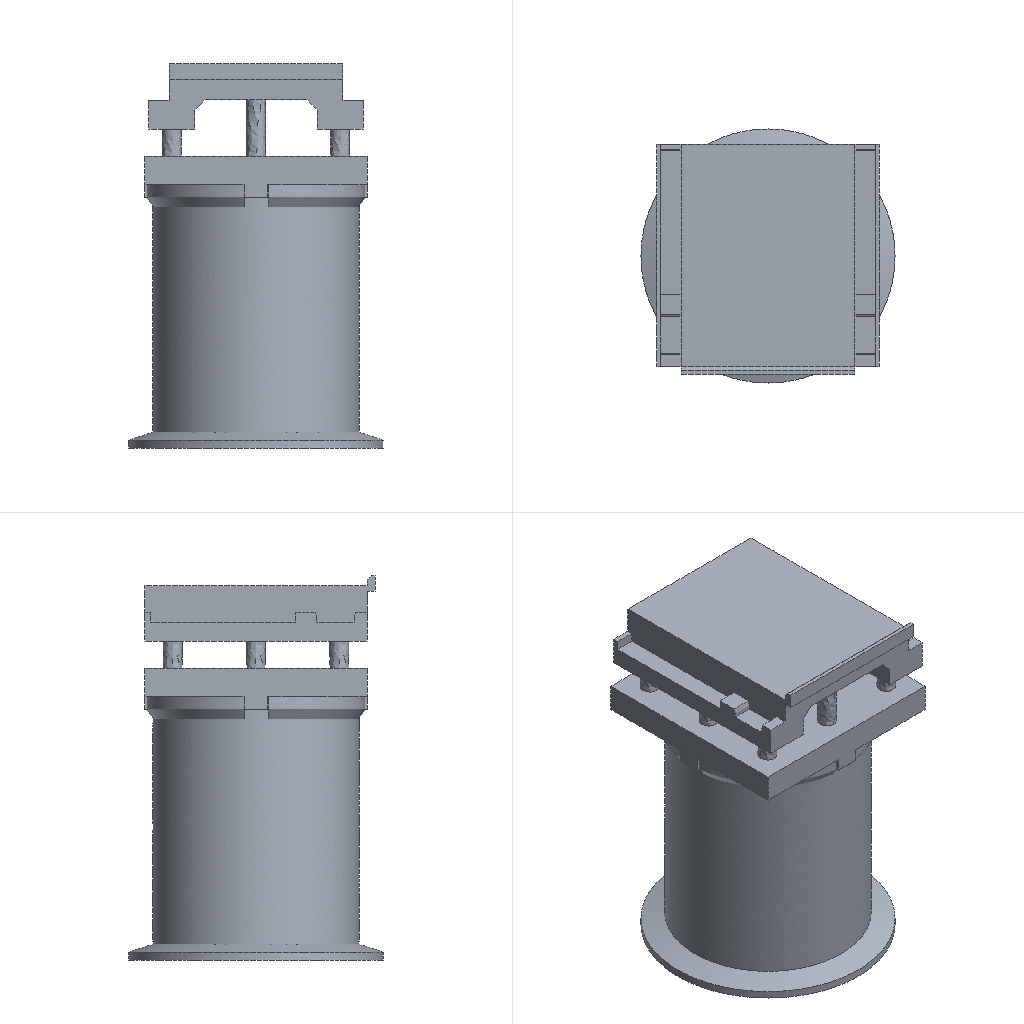Simulation study | ansys workbench
Ansys APDL input file, long lists of numbers shortened:
/batch
/config,noeldb,1     ! force off writing results to database
*get,_wallstrt,active,,time,wall
! ANSYS input file written by Workbench version 2022 R1
! File used for geometry attach:
/title,wbnew--____ (A5)
! ****** Begin Custom Load Command Snippet ******
/COM, ACT Extensions:
/COM,     LSDYNA, 2021.1
/COM,
! ****** End   Custom Load Command Snippet ******
*DIM,_wb_ProjectScratch_dir,string,248
_wb_ProjectScratch_dir(1) = ''
*DIM,_wb_SolverFiles_dir,string,248
_wb_SolverFiles_dir(1) = ''
*DIM,_wb_userfiles_dir,string,248
_wb_userfiles_dir(1) = ''
/com,--- Data in consistent MKS units. See Solving Units in the help system for more information.
/units,MKS
/nopr
/wb,file,start              !  signify a WB generated input file
/prep7
! Turn off shape checking because checks already performed inside WB mesher.
! See help system for more information.
SHPP,OFF,,NOWARN
/nolist
etcon,set             ! allow ANSYS to choose best KEYOP's for 180x elements, resets any applicable keyopt to MAPDL defaults
/com,*********** Nodes for the whole assembly ***********
nblock,3,,165333
(1i9,3e20.9e3)
        1    -4.091861413E+02     3.968814041E+01    -2.039000000E+01
! (150302 more lines like these left out)
-1
/wb,elem,start            !  set before creation of elements
/com,*********** Elements for Body 1 "a953f0-7" ***********
et,1,187
eblock,19,solid,,87505
(19i9)
        1        1        1        1        0        0        0        0       10        0        1    11820    23372    11975    23358    91085    91919    91082    91084
! (175009 more lines like these left out)
-1
/wb,elem,end               !  done creating elements
/com,*********** Send User Defined Coordinate System(s) ***********
csys,0
toffst,273.15,  ! Temperature offset from absolute zero
/com,*********** Set Reference Temperature ***********
tref,22.
/wb,mat,start              !  starting to send materials
/com,*********** Send Materials ***********
Temperature = 'TEMP' ! Temperature
MP,DENS,1,2300,	! kg m^-3
MP,ALPX,1,1.4e-05,	! C^-1
MP,C,1,780,	! J kg^-1 C^-1
MP,KXX,1,0.72,	! W m^-1 C^-1
MP,EX,1,30000000000,	! Pa
MP,NUXY,1,0.18,
/wb,mat,end                !  done sending materials
!************************* Model Summary ********************
!a953f0-7,	混凝土,	matid,	1
!************************* End Model Summary ********************
! get the diagonal of the bounding box. Needed later for other things
*get,_xmin,node,,mnloc,x
*get,_ymin,node,,mnloc,y
*get,_zmin,node,,mnloc,z
*get,_xmax,node,,mxloc,x
*get,_ymax,node,,mxloc,y
*get,_zmax,node,,mxloc,z
_ASMDIAG=(_xmax-_xmin)*(_xmax-_xmin)+(_ymax-_ymin)*(_ymax-_ymin)+(_zmax-_zmin)*(_zmax-_zmin)
_ASMDIAG=SQRT(_ASMDIAG)
/wb,contact,start          !  starting to send contact
/wb,contact,end            !  done creating contacts
/golist
/wb,load,start             !  starting to send loads
/com,*********** Fixed Supports ***********
CMBLOCK,_FIXEDSU,NODE,     7355
(8i10)
         1        96       121       122       123       124       125       126
! (919 more lines like these left out)
cmsel,s,_FIXEDSU
d,all,all
nsel,all
/com,*********** Define Force Using Surface Effect Elements ***********
local,12,0,0.,0.,0.,0.,0.,0.
csys,0
et,2,154
eblock,10,,,7449
(15i9)
   119600        2        2        2       12       15    11737       14       14    23478    23472       14    23468
! (7448 more lines like these left out)
-1
esel,s,type,,2
keyop,2,2,1                ! Apply load in local coordinate system
keyop,2,7,1                ! Use original area so load is constant in large deformation
esel,all
/gst,on,on
fini
*get,_numnode,node,0,count
*get,_numelem,elem,0,count
*get, _MAXELEMNUM, elem, 0, NUM, MAX
*get, _MAXNODENUM, node, 0, NUM, MAX
*get, _MAXELEMTYPE, etyp, 0, NUM, MAX
*get, _MAXREALCONST, real, 0, NUM, MAX
/go
/wb,load,end               !  done creating loads
/com,--- Number of total nodes = %_numnode%
/com,--- Number of contact elements = 7449
/com,--- Number of spring elements = 0
/com,--- Number of bearing elements = 0
/com,--- Number of solid elements = 87505
/com,--- Number of condensed parts = 0
/com,--- Number of total elements = %_numelem%
*get,_wallbsol,active,,time,wall
/com,****************************************************************************
/com,*************************    SOLUTION       ********************************
/com,****************************************************************************
/solu
antype,0                   ! static analysis
_thickRatio=  1     ! Ratio of thick parts in the model
eqsl,pcg,1e-8,,,,,,1
cntr,print,1               ! print out contact info and also make no initial contact an error
dmpoption,emat,no             ! Don't combine emat file for DANSYS
dmpoption,esav,no             ! Don't combine esav file for DANSYS
nldiag,cont,iter           ! print out contact info each equilibrium iteration
rescontrol,,none                 ! Do not keep any restart files
/com,****************************************************
/com,******************* SOLVE FOR LS 1 OF 1 ****************
esel,s,type,,2
nsle
sfe,all,1,pres,1,0.
sfe,all,2,pres,1,-21371.338
sfe,all,3,pres,1,0.
nsel,all
esel,all
acel,0.,0.,9.807
/nopr
/gopr
nsub,1,1,1
time,1.e-002
outres,erase
outres,all,none
outres,nsol,all,
outres,rsol,all
outres,eangl,all
outres,etmp,all
outres,veng,all
outres,strs,all,
outres,epel,all,
outres,eppl,all,
outres,cont,all,
! *********** WB SOLVE COMMAND ***********
! check interactive state
*get,ANSINTER_,active,,int
*if,ANSINTER_,ne,0,then
/eof
*endif
solve
/com *************** Write FE CONNECTORS *********
CEWRITE,file,ce,,INTE
/com,****************************************************
/com,*************** FINISHED SOLVE FOR LS 1 *************
*get,_wallasol,active,,time,wall
/nopr
*get,_numnode,node,0,count
*get,_numelem,elem,0,count
*get, _MAXELEMNUM, elem, 0, NUM, MAX
*get, _MAXNODENUM, node, 0, NUM, MAX,,,INTERNAL
*get, _MAXELEMTYPE, etyp, 0, NUM, MAX
*get, _MAXREALCONST, real, 0, NUM, MAX
/gopr
*get,_PCGITER,active,,solu,cgiter
/post1
xmlo,ENCODING,ISO-8859-1
xmlo,parm
/xml,parm,xml
fini
/gopr
*get,_walldone,active,,time,wall
_preptime=(_wallbsol-_wallstrt)*3600
_solvtime=(_wallasol-_wallbsol)*3600
_posttime=(_walldone-_wallasol)*3600
_totaltim=(_walldone-_wallstrt)*3600
*get,_dlbratio,active,0,solu,dlbr
*get,_combtime,active,0,solu,comb
*get,_ssmode,active,0,solu,ssmm
*get,_ndofs,active,0,solu,ndof
*get,_sol_end_time,active,0,set,time
*if,_sol_end_time,eq,0.01,then
/fclean				!clean distributed files
*endif
/com,--- Total number of nodes = %_numnode%
/com,--- Total number of elements = %_numelem%
/com,--- Element load balance ratio = %_dlbratio%
/com,--- Time to combine distributed files = %_combtime%
/com,--- Sparse memory mode = %_ssmode%
/com,--- Number of DOF = %_ndofs%
/wb,file,end               ! done with WB generated input